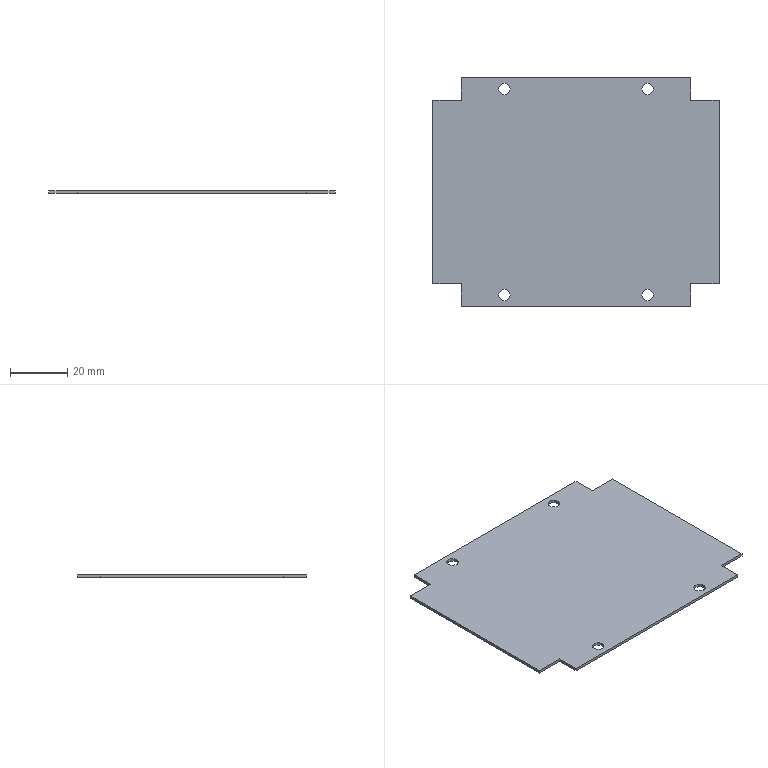Part | SolidWorks | features Extrusion 1 | 1 solid | 22 faces | box 100 x 80 x 1 mm | volume 7630 mm3 | plane 14 | cylinder 8 | commonest cylinder face diameters 4 x8
STEP:
#1=CARTESIAN_POINT('',(23.,-36.,1.));
#2=VERTEX_POINT('',#1);
#3=CARTESIAN_POINT('',(27.,-36.,1.));
#4=VERTEX_POINT('',#3);
#5=CARTESIAN_POINT('',(25.,-36.,1.));
#6=DIRECTION('',(0.,0.,1.));
#7=DIRECTION('',(1.,0.,0.));
#8=AXIS2_PLACEMENT_3D('',#5,#6,#7);
#9=CIRCLE('',#8,2.);
#10=EDGE_CURVE('',#2,#4,#9,.T.);
#11=ORIENTED_EDGE('',*,*,#10,.T.);
#12=CARTESIAN_POINT('',(27.,-36.,0.));
#13=VERTEX_POINT('',#12);
#14=CARTESIAN_POINT('',(27.,-36.,1.));
#15=DIRECTION('',(0.,0.,-1.));
#16=VECTOR('',#15,1000.);
#17=LINE('',#14,#16);
#18=EDGE_CURVE('',#4,#13,#17,.T.);
#19=ORIENTED_EDGE('',*,*,#18,.T.);
#20=CARTESIAN_POINT('',(23.,-36.,0.));
#21=VERTEX_POINT('',#20);
#22=CARTESIAN_POINT('',(25.,-36.,0.));
#23=DIRECTION('',(0.,0.,1.));
#24=DIRECTION('',(1.,0.,0.));
#25=AXIS2_PLACEMENT_3D('',#22,#23,#24);
#26=CIRCLE('',#25,2.);
#27=EDGE_CURVE('',#21,#13,#26,.T.);
#28=ORIENTED_EDGE('',*,*,#27,.F.);
#29=CARTESIAN_POINT('',(23.,-36.,1.));
#30=DIRECTION('',(0.,0.,-1.));
#31=VECTOR('',#30,1000.);
#32=LINE('',#29,#31);
#33=EDGE_CURVE('',#2,#21,#32,.T.);
#34=ORIENTED_EDGE('',*,*,#33,.F.);
#35=EDGE_LOOP('',(#11,#19,#28,#34));
#36=FACE_OUTER_BOUND('',#35,.T.);
#37=CARTESIAN_POINT('',(25.,-36.,1.));
#38=DIRECTION('',(0.,0.,-1.));
#39=DIRECTION('',(-1.,0.,0.));
#40=AXIS2_PLACEMENT_3D('',#37,#38,#39);
#41=CYLINDRICAL_SURFACE('',#40,2.);
#42=ADVANCED_FACE('',(#36),#41,.F.);
#43=CARTESIAN_POINT('',(23.,36.,1.));
#44=VERTEX_POINT('',#43);
#45=CARTESIAN_POINT('',(27.,36.,1.));
#46=VERTEX_POINT('',#45);
#47=CARTESIAN_POINT('',(25.,36.,1.));
#48=DIRECTION('',(0.,0.,1.));
#49=DIRECTION('',(1.,0.,0.));
#50=AXIS2_PLACEMENT_3D('',#47,#48,#49);
#51=CIRCLE('',#50,2.);
#52=EDGE_CURVE('',#44,#46,#51,.T.);
#53=ORIENTED_EDGE('',*,*,#52,.T.);
#54=CARTESIAN_POINT('',(27.,36.,0.));
#55=VERTEX_POINT('',#54);
#56=CARTESIAN_POINT('',(27.,36.,1.));
#57=DIRECTION('',(0.,0.,-1.));
#58=VECTOR('',#57,1000.);
#59=LINE('',#56,#58);
#60=EDGE_CURVE('',#46,#55,#59,.T.);
#61=ORIENTED_EDGE('',*,*,#60,.T.);
#62=CARTESIAN_POINT('',(23.,36.,0.));
#63=VERTEX_POINT('',#62);
#64=CARTESIAN_POINT('',(25.,36.,0.));
#65=DIRECTION('',(0.,0.,1.));
#66=DIRECTION('',(1.,0.,0.));
#67=AXIS2_PLACEMENT_3D('',#64,#65,#66);
#68=CIRCLE('',#67,2.);
#69=EDGE_CURVE('',#63,#55,#68,.T.);
#70=ORIENTED_EDGE('',*,*,#69,.F.);
#71=CARTESIAN_POINT('',(23.,36.,1.));
#72=DIRECTION('',(0.,0.,-1.));
#73=VECTOR('',#72,1000.);
#74=LINE('',#71,#73);
#75=EDGE_CURVE('',#44,#63,#74,.T.);
#76=ORIENTED_EDGE('',*,*,#75,.F.);
#77=EDGE_LOOP('',(#53,#61,#70,#76));
#78=FACE_OUTER_BOUND('',#77,.T.);
#79=CARTESIAN_POINT('',(25.,36.,1.));
#80=DIRECTION('',(0.,0.,-1.));
#81=DIRECTION('',(-1.,0.,0.));
#82=AXIS2_PLACEMENT_3D('',#79,#80,#81);
#83=CYLINDRICAL_SURFACE('',#82,2.);
#84=ADVANCED_FACE('',(#78),#83,.F.);
#85=CARTESIAN_POINT('',(-27.,-36.,1.));
#86=VERTEX_POINT('',#85);
#87=CARTESIAN_POINT('',(-23.,-36.,1.));
#88=VERTEX_POINT('',#87);
#89=CARTESIAN_POINT('',(-25.,-36.,1.));
#90=DIRECTION('',(0.,0.,1.));
#91=DIRECTION('',(1.,0.,0.));
#92=AXIS2_PLACEMENT_3D('',#89,#90,#91);
#93=CIRCLE('',#92,2.);
#94=EDGE_CURVE('',#86,#88,#93,.T.);
#95=ORIENTED_EDGE('',*,*,#94,.T.);
#96=CARTESIAN_POINT('',(-23.,-36.,0.));
#97=VERTEX_POINT('',#96);
#98=CARTESIAN_POINT('',(-23.,-36.,1.));
#99=DIRECTION('',(0.,0.,-1.));
#100=VECTOR('',#99,1000.);
#101=LINE('',#98,#100);
#102=EDGE_CURVE('',#88,#97,#101,.T.);
#103=ORIENTED_EDGE('',*,*,#102,.T.);
#104=CARTESIAN_POINT('',(-27.,-36.,0.));
#105=VERTEX_POINT('',#104);
#106=CARTESIAN_POINT('',(-25.,-36.,0.));
#107=DIRECTION('',(0.,0.,1.));
#108=DIRECTION('',(1.,0.,0.));
#109=AXIS2_PLACEMENT_3D('',#106,#107,#108);
#110=CIRCLE('',#109,2.);
#111=EDGE_CURVE('',#105,#97,#110,.T.);
#112=ORIENTED_EDGE('',*,*,#111,.F.);
#113=CARTESIAN_POINT('',(-27.,-36.,1.));
#114=DIRECTION('',(0.,0.,-1.));
#115=VECTOR('',#114,1000.);
#116=LINE('',#113,#115);
#117=EDGE_CURVE('',#86,#105,#116,.T.);
#118=ORIENTED_EDGE('',*,*,#117,.F.);
#119=EDGE_LOOP('',(#95,#103,#112,#118));
#120=FACE_OUTER_BOUND('',#119,.T.);
#121=CARTESIAN_POINT('',(-25.,-36.,1.));
#122=DIRECTION('',(0.,0.,-1.));
#123=DIRECTION('',(-1.,0.,0.));
#124=AXIS2_PLACEMENT_3D('',#121,#122,#123);
#125=CYLINDRICAL_SURFACE('',#124,2.);
#126=ADVANCED_FACE('',(#120),#125,.F.);
#127=CARTESIAN_POINT('',(-27.,36.,1.));
#128=VERTEX_POINT('',#127);
#129=CARTESIAN_POINT('',(-23.,36.,1.));
#130=VERTEX_POINT('',#129);
#131=CARTESIAN_POINT('',(-25.,36.,1.));
#132=DIRECTION('',(0.,0.,1.));
#133=DIRECTION('',(1.,0.,0.));
#134=AXIS2_PLACEMENT_3D('',#131,#132,#133);
#135=CIRCLE('',#134,2.);
#136=EDGE_CURVE('',#128,#130,#135,.T.);
#137=ORIENTED_EDGE('',*,*,#136,.T.);
#138=CARTESIAN_POINT('',(-23.,36.,0.));
#139=VERTEX_POINT('',#138);
#140=CARTESIAN_POINT('',(-23.,36.,1.));
#141=DIRECTION('',(0.,0.,-1.));
#142=VECTOR('',#141,1000.);
#143=LINE('',#140,#142);
#144=EDGE_CURVE('',#130,#139,#143,.T.);
#145=ORIENTED_EDGE('',*,*,#144,.T.);
#146=CARTESIAN_POINT('',(-27.,36.,0.));
#147=VERTEX_POINT('',#146);
#148=CARTESIAN_POINT('',(-25.,36.,0.));
#149=DIRECTION('',(0.,0.,1.));
#150=DIRECTION('',(1.,0.,0.));
#151=AXIS2_PLACEMENT_3D('',#148,#149,#150);
#152=CIRCLE('',#151,2.);
#153=EDGE_CURVE('',#147,#139,#152,.T.);
#154=ORIENTED_EDGE('',*,*,#153,.F.);
#155=CARTESIAN_POINT('',(-27.,36.,1.));
#156=DIRECTION('',(0.,0.,-1.));
#157=VECTOR('',#156,1000.);
#158=LINE('',#155,#157);
#159=EDGE_CURVE('',#128,#147,#158,.T.);
#160=ORIENTED_EDGE('',*,*,#159,.F.);
#161=EDGE_LOOP('',(#137,#145,#154,#160));
#162=FACE_OUTER_BOUND('',#161,.T.);
#163=CARTESIAN_POINT('',(-25.,36.,1.));
#164=DIRECTION('',(0.,0.,-1.));
#165=DIRECTION('',(-1.,0.,0.));
#166=AXIS2_PLACEMENT_3D('',#163,#164,#165);
#167=CYLINDRICAL_SURFACE('',#166,2.);
#168=ADVANCED_FACE('',(#162),#167,.F.);
#169=ORIENTED_EDGE('',*,*,#52,.F.);
#170=CARTESIAN_POINT('',(25.,36.,1.));
#171=DIRECTION('',(0.,0.,1.));
#172=DIRECTION('',(1.,0.,0.));
#173=AXIS2_PLACEMENT_3D('',#170,#171,#172);
#174=CIRCLE('',#173,2.);
#175=EDGE_CURVE('',#46,#44,#174,.T.);
#176=ORIENTED_EDGE('',*,*,#175,.F.);
#177=EDGE_LOOP('',(#169,#176));
#178=FACE_BOUND('',#177,.T.);
#179=ORIENTED_EDGE('',*,*,#136,.F.);
#180=CARTESIAN_POINT('',(-25.,36.,1.));
#181=DIRECTION('',(0.,0.,1.));
#182=DIRECTION('',(1.,0.,0.));
#183=AXIS2_PLACEMENT_3D('',#180,#181,#182);
#184=CIRCLE('',#183,2.);
#185=EDGE_CURVE('',#130,#128,#184,.T.);
#186=ORIENTED_EDGE('',*,*,#185,.F.);
#187=EDGE_LOOP('',(#179,#186));
#188=FACE_BOUND('',#187,.T.);
#189=CARTESIAN_POINT('',(-40.,32.,1.));
#190=VERTEX_POINT('',#189);
#191=CARTESIAN_POINT('',(-50.,32.,1.));
#192=VERTEX_POINT('',#191);
#193=CARTESIAN_POINT('',(-50.,32.,1.));
#194=DIRECTION('',(-1.,0.,0.));
#195=VECTOR('',#194,1000.);
#196=LINE('',#193,#195);
#197=EDGE_CURVE('',#190,#192,#196,.T.);
#198=ORIENTED_EDGE('',*,*,#197,.T.);
#199=CARTESIAN_POINT('',(-50.,-32.,1.));
#200=VERTEX_POINT('',#199);
#201=CARTESIAN_POINT('',(-50.,32.,1.));
#202=DIRECTION('',(0.,-1.,0.));
#203=VECTOR('',#202,1000.);
#204=LINE('',#201,#203);
#205=EDGE_CURVE('',#192,#200,#204,.T.);
#206=ORIENTED_EDGE('',*,*,#205,.T.);
#207=CARTESIAN_POINT('',(-40.,-32.,1.));
#208=VERTEX_POINT('',#207);
#209=CARTESIAN_POINT('',(-50.,-32.,1.));
#210=DIRECTION('',(1.,0.,0.));
#211=VECTOR('',#210,1000.);
#212=LINE('',#209,#211);
#213=EDGE_CURVE('',#200,#208,#212,.T.);
#214=ORIENTED_EDGE('',*,*,#213,.T.);
#215=CARTESIAN_POINT('',(-40.,-40.,1.));
#216=VERTEX_POINT('',#215);
#217=CARTESIAN_POINT('',(-40.,-32.,1.));
#218=DIRECTION('',(0.,-1.,0.));
#219=VECTOR('',#218,1000.);
#220=LINE('',#217,#219);
#221=EDGE_CURVE('',#208,#216,#220,.T.);
#222=ORIENTED_EDGE('',*,*,#221,.T.);
#223=CARTESIAN_POINT('',(40.,-40.,1.));
#224=VERTEX_POINT('',#223);
#225=CARTESIAN_POINT('',(-40.,-40.,1.));
#226=DIRECTION('',(1.,0.,0.));
#227=VECTOR('',#226,1000.);
#228=LINE('',#225,#227);
#229=EDGE_CURVE('',#216,#224,#228,.T.);
#230=ORIENTED_EDGE('',*,*,#229,.T.);
#231=CARTESIAN_POINT('',(40.,-32.,1.));
#232=VERTEX_POINT('',#231);
#233=CARTESIAN_POINT('',(40.,-32.,1.));
#234=DIRECTION('',(0.,1.,0.));
#235=VECTOR('',#234,1000.);
#236=LINE('',#233,#235);
#237=EDGE_CURVE('',#224,#232,#236,.T.);
#238=ORIENTED_EDGE('',*,*,#237,.T.);
#239=CARTESIAN_POINT('',(50.,-32.,1.));
#240=VERTEX_POINT('',#239);
#241=CARTESIAN_POINT('',(50.,-32.,1.));
#242=DIRECTION('',(1.,0.,0.));
#243=VECTOR('',#242,1000.);
#244=LINE('',#241,#243);
#245=EDGE_CURVE('',#232,#240,#244,.T.);
#246=ORIENTED_EDGE('',*,*,#245,.T.);
#247=CARTESIAN_POINT('',(50.,32.,1.));
#248=VERTEX_POINT('',#247);
#249=CARTESIAN_POINT('',(50.,32.,1.));
#250=DIRECTION('',(0.,1.,0.));
#251=VECTOR('',#250,1000.);
#252=LINE('',#249,#251);
#253=EDGE_CURVE('',#240,#248,#252,.T.);
#254=ORIENTED_EDGE('',*,*,#253,.T.);
#255=CARTESIAN_POINT('',(40.,32.,1.));
#256=VERTEX_POINT('',#255);
#257=CARTESIAN_POINT('',(50.,32.,1.));
#258=DIRECTION('',(-1.,0.,0.));
#259=VECTOR('',#258,1000.);
#260=LINE('',#257,#259);
#261=EDGE_CURVE('',#248,#256,#260,.T.);
#262=ORIENTED_EDGE('',*,*,#261,.T.);
#263=CARTESIAN_POINT('',(40.,40.,1.));
#264=VERTEX_POINT('',#263);
#265=CARTESIAN_POINT('',(40.,32.,1.));
#266=DIRECTION('',(0.,1.,0.));
#267=VECTOR('',#266,1000.);
#268=LINE('',#265,#267);
#269=EDGE_CURVE('',#256,#264,#268,.T.);
#270=ORIENTED_EDGE('',*,*,#269,.T.);
#271=CARTESIAN_POINT('',(-40.,40.,1.));
#272=VERTEX_POINT('',#271);
#273=CARTESIAN_POINT('',(-40.,40.,1.));
#274=DIRECTION('',(-1.,0.,0.));
#275=VECTOR('',#274,1000.);
#276=LINE('',#273,#275);
#277=EDGE_CURVE('',#264,#272,#276,.T.);
#278=ORIENTED_EDGE('',*,*,#277,.T.);
#279=CARTESIAN_POINT('',(-40.,32.,1.));
#280=DIRECTION('',(0.,-1.,0.));
#281=VECTOR('',#280,1000.);
#282=LINE('',#279,#281);
#283=EDGE_CURVE('',#272,#190,#282,.T.);
#284=ORIENTED_EDGE('',*,*,#283,.T.);
#285=EDGE_LOOP('',(#198,#206,#214,#222,#230,#238,#246,#254,#262,#270,#278,#284));
#286=FACE_OUTER_BOUND('',#285,.T.);
#287=ORIENTED_EDGE('',*,*,#94,.F.);
#288=CARTESIAN_POINT('',(-25.,-36.,1.));
#289=DIRECTION('',(0.,0.,1.));
#290=DIRECTION('',(1.,0.,0.));
#291=AXIS2_PLACEMENT_3D('',#288,#289,#290);
#292=CIRCLE('',#291,2.);
#293=EDGE_CURVE('',#88,#86,#292,.T.);
#294=ORIENTED_EDGE('',*,*,#293,.F.);
#295=EDGE_LOOP('',(#287,#294));
#296=FACE_BOUND('',#295,.T.);
#297=ORIENTED_EDGE('',*,*,#10,.F.);
#298=CARTESIAN_POINT('',(25.,-36.,1.));
#299=DIRECTION('',(0.,0.,1.));
#300=DIRECTION('',(1.,0.,0.));
#301=AXIS2_PLACEMENT_3D('',#298,#299,#300);
#302=CIRCLE('',#301,2.);
#303=EDGE_CURVE('',#4,#2,#302,.T.);
#304=ORIENTED_EDGE('',*,*,#303,.F.);
#305=EDGE_LOOP('',(#297,#304));
#306=FACE_BOUND('',#305,.T.);
#307=CARTESIAN_POINT('',(0.,0.,1.));
#308=DIRECTION('',(0.,0.,1.));
#309=DIRECTION('',(1.,0.,0.));
#310=AXIS2_PLACEMENT_3D('',#307,#308,#309);
#311=PLANE('',#310);
#312=ADVANCED_FACE('',(#178,#188,#286,#296,#306),#311,.T.);
#313=CARTESIAN_POINT('',(-40.,32.,0.));
#314=VERTEX_POINT('',#313);
#315=CARTESIAN_POINT('',(-50.,32.,0.));
#316=VERTEX_POINT('',#315);
#317=CARTESIAN_POINT('',(-50.,32.,0.));
#318=DIRECTION('',(-1.,0.,0.));
#319=VECTOR('',#318,1000.);
#320=LINE('',#317,#319);
#321=EDGE_CURVE('',#314,#316,#320,.T.);
#322=ORIENTED_EDGE('',*,*,#321,.F.);
#323=CARTESIAN_POINT('',(-40.,40.,0.));
#324=VERTEX_POINT('',#323);
#325=CARTESIAN_POINT('',(-40.,32.,0.));
#326=DIRECTION('',(0.,-1.,0.));
#327=VECTOR('',#326,1000.);
#328=LINE('',#325,#327);
#329=EDGE_CURVE('',#324,#314,#328,.T.);
#330=ORIENTED_EDGE('',*,*,#329,.F.);
#331=CARTESIAN_POINT('',(40.,40.,0.));
#332=VERTEX_POINT('',#331);
#333=CARTESIAN_POINT('',(-40.,40.,0.));
#334=DIRECTION('',(-1.,0.,0.));
#335=VECTOR('',#334,1000.);
#336=LINE('',#333,#335);
#337=EDGE_CURVE('',#332,#324,#336,.T.);
#338=ORIENTED_EDGE('',*,*,#337,.F.);
#339=CARTESIAN_POINT('',(40.,32.,0.));
#340=VERTEX_POINT('',#339);
#341=CARTESIAN_POINT('',(40.,32.,0.));
#342=DIRECTION('',(0.,1.,0.));
#343=VECTOR('',#342,1000.);
#344=LINE('',#341,#343);
#345=EDGE_CURVE('',#340,#332,#344,.T.);
#346=ORIENTED_EDGE('',*,*,#345,.F.);
#347=CARTESIAN_POINT('',(50.,32.,0.));
#348=VERTEX_POINT('',#347);
#349=CARTESIAN_POINT('',(50.,32.,0.));
#350=DIRECTION('',(-1.,0.,0.));
#351=VECTOR('',#350,1000.);
#352=LINE('',#349,#351);
#353=EDGE_CURVE('',#348,#340,#352,.T.);
#354=ORIENTED_EDGE('',*,*,#353,.F.);
#355=CARTESIAN_POINT('',(50.,-32.,0.));
#356=VERTEX_POINT('',#355);
#357=CARTESIAN_POINT('',(50.,32.,0.));
#358=DIRECTION('',(0.,1.,0.));
#359=VECTOR('',#358,1000.);
#360=LINE('',#357,#359);
#361=EDGE_CURVE('',#356,#348,#360,.T.);
#362=ORIENTED_EDGE('',*,*,#361,.F.);
#363=CARTESIAN_POINT('',(40.,-32.,0.));
#364=VERTEX_POINT('',#363);
#365=CARTESIAN_POINT('',(50.,-32.,0.));
#366=DIRECTION('',(1.,0.,0.));
#367=VECTOR('',#366,1000.);
#368=LINE('',#365,#367);
#369=EDGE_CURVE('',#364,#356,#368,.T.);
#370=ORIENTED_EDGE('',*,*,#369,.F.);
#371=CARTESIAN_POINT('',(40.,-40.,0.));
#372=VERTEX_POINT('',#371);
#373=CARTESIAN_POINT('',(40.,-32.,0.));
#374=DIRECTION('',(0.,1.,0.));
#375=VECTOR('',#374,1000.);
#376=LINE('',#373,#375);
#377=EDGE_CURVE('',#372,#364,#376,.T.);
#378=ORIENTED_EDGE('',*,*,#377,.F.);
#379=CARTESIAN_POINT('',(-40.,-40.,0.));
#380=VERTEX_POINT('',#379);
#381=CARTESIAN_POINT('',(-40.,-40.,0.));
#382=DIRECTION('',(1.,0.,0.));
#383=VECTOR('',#382,1000.);
#384=LINE('',#381,#383);
#385=EDGE_CURVE('',#380,#372,#384,.T.);
#386=ORIENTED_EDGE('',*,*,#385,.F.);
#387=CARTESIAN_POINT('',(-40.,-32.,0.));
#388=VERTEX_POINT('',#387);
#389=CARTESIAN_POINT('',(-40.,-32.,0.));
#390=DIRECTION('',(0.,-1.,0.));
#391=VECTOR('',#390,1000.);
#392=LINE('',#389,#391);
#393=EDGE_CURVE('',#388,#380,#392,.T.);
#394=ORIENTED_EDGE('',*,*,#393,.F.);
#395=CARTESIAN_POINT('',(-50.,-32.,0.));
#396=VERTEX_POINT('',#395);
#397=CARTESIAN_POINT('',(-50.,-32.,0.));
#398=DIRECTION('',(1.,0.,0.));
#399=VECTOR('',#398,1000.);
#400=LINE('',#397,#399);
#401=EDGE_CURVE('',#396,#388,#400,.T.);
#402=ORIENTED_EDGE('',*,*,#401,.F.);
#403=CARTESIAN_POINT('',(-50.,32.,0.));
#404=DIRECTION('',(0.,-1.,0.));
#405=VECTOR('',#404,1000.);
#406=LINE('',#403,#405);
#407=EDGE_CURVE('',#316,#396,#406,.T.);
#408=ORIENTED_EDGE('',*,*,#407,.F.);
#409=EDGE_LOOP('',(#322,#330,#338,#346,#354,#362,#370,#378,#386,#394,#402,#408));
#410=FACE_OUTER_BOUND('',#409,.T.);
#411=ORIENTED_EDGE('',*,*,#153,.T.);
#412=CARTESIAN_POINT('',(-25.,36.,0.));
#413=DIRECTION('',(0.,0.,1.));
#414=DIRECTION('',(1.,0.,0.));
#415=AXIS2_PLACEMENT_3D('',#412,#413,#414);
#416=CIRCLE('',#415,2.);
#417=EDGE_CURVE('',#139,#147,#416,.T.);
#418=ORIENTED_EDGE('',*,*,#417,.T.);
#419=EDGE_LOOP('',(#411,#418));
#420=FACE_BOUND('',#419,.T.);
#421=ORIENTED_EDGE('',*,*,#111,.T.);
#422=CARTESIAN_POINT('',(-25.,-36.,0.));
#423=DIRECTION('',(0.,0.,1.));
#424=DIRECTION('',(1.,0.,0.));
#425=AXIS2_PLACEMENT_3D('',#422,#423,#424);
#426=CIRCLE('',#425,2.);
#427=EDGE_CURVE('',#97,#105,#426,.T.);
#428=ORIENTED_EDGE('',*,*,#427,.T.);
#429=EDGE_LOOP('',(#421,#428));
#430=FACE_BOUND('',#429,.T.);
#431=ORIENTED_EDGE('',*,*,#69,.T.);
#432=CARTESIAN_POINT('',(25.,36.,0.));
#433=DIRECTION('',(0.,0.,1.));
#434=DIRECTION('',(1.,0.,0.));
#435=AXIS2_PLACEMENT_3D('',#432,#433,#434);
#436=CIRCLE('',#435,2.);
#437=EDGE_CURVE('',#55,#63,#436,.T.);
#438=ORIENTED_EDGE('',*,*,#437,.T.);
#439=EDGE_LOOP('',(#431,#438));
#440=FACE_BOUND('',#439,.T.);
#441=ORIENTED_EDGE('',*,*,#27,.T.);
#442=CARTESIAN_POINT('',(25.,-36.,0.));
#443=DIRECTION('',(0.,0.,1.));
#444=DIRECTION('',(1.,0.,0.));
#445=AXIS2_PLACEMENT_3D('',#442,#443,#444);
#446=CIRCLE('',#445,2.);
#447=EDGE_CURVE('',#13,#21,#446,.T.);
#448=ORIENTED_EDGE('',*,*,#447,.T.);
#449=EDGE_LOOP('',(#441,#448));
#450=FACE_BOUND('',#449,.T.);
#451=CARTESIAN_POINT('',(0.,0.,0.));
#452=DIRECTION('',(0.,0.,1.));
#453=DIRECTION('',(1.,0.,0.));
#454=AXIS2_PLACEMENT_3D('',#451,#452,#453);
#455=PLANE('',#454);
#456=ADVANCED_FACE('',(#410,#420,#430,#440,#450),#455,.F.);
#457=ORIENTED_EDGE('',*,*,#321,.T.);
#458=CARTESIAN_POINT('',(-50.,32.,1.));
#459=DIRECTION('',(0.,0.,-1.));
#460=VECTOR('',#459,1000.);
#461=LINE('',#458,#460);
#462=EDGE_CURVE('',#192,#316,#461,.T.);
#463=ORIENTED_EDGE('',*,*,#462,.F.);
#464=ORIENTED_EDGE('',*,*,#197,.F.);
#465=CARTESIAN_POINT('',(-40.,32.,1.));
#466=DIRECTION('',(0.,0.,-1.));
#467=VECTOR('',#466,1000.);
#468=LINE('',#465,#467);
#469=EDGE_CURVE('',#190,#314,#468,.T.);
#470=ORIENTED_EDGE('',*,*,#469,.T.);
#471=EDGE_LOOP('',(#457,#463,#464,#470));
#472=FACE_OUTER_BOUND('',#471,.T.);
#473=CARTESIAN_POINT('',(-50.,32.,1.));
#474=DIRECTION('',(0.,-1.,0.));
#475=DIRECTION('',(0.,0.,-1.));
#476=AXIS2_PLACEMENT_3D('',#473,#474,#475);
#477=PLANE('',#476);
#478=ADVANCED_FACE('',(#472),#477,.F.);
#479=ORIENTED_EDGE('',*,*,#407,.T.);
#480=CARTESIAN_POINT('',(-50.,-32.,1.));
#481=DIRECTION('',(0.,0.,-1.));
#482=VECTOR('',#481,1000.);
#483=LINE('',#480,#482);
#484=EDGE_CURVE('',#200,#396,#483,.T.);
#485=ORIENTED_EDGE('',*,*,#484,.F.);
#486=ORIENTED_EDGE('',*,*,#205,.F.);
#487=ORIENTED_EDGE('',*,*,#462,.T.);
#488=EDGE_LOOP('',(#479,#485,#486,#487));
#489=FACE_OUTER_BOUND('',#488,.T.);
#490=CARTESIAN_POINT('',(-50.,32.,1.));
#491=DIRECTION('',(1.,0.,0.));
#492=DIRECTION('',(0.,1.,0.));
#493=AXIS2_PLACEMENT_3D('',#490,#491,#492);
#494=PLANE('',#493);
#495=ADVANCED_FACE('',(#489),#494,.F.);
#496=ORIENTED_EDGE('',*,*,#401,.T.);
#497=CARTESIAN_POINT('',(-40.,-32.,1.));
#498=DIRECTION('',(0.,0.,-1.));
#499=VECTOR('',#498,1000.);
#500=LINE('',#497,#499);
#501=EDGE_CURVE('',#208,#388,#500,.T.);
#502=ORIENTED_EDGE('',*,*,#501,.F.);
#503=ORIENTED_EDGE('',*,*,#213,.F.);
#504=ORIENTED_EDGE('',*,*,#484,.T.);
#505=EDGE_LOOP('',(#496,#502,#503,#504));
#506=FACE_OUTER_BOUND('',#505,.T.);
#507=CARTESIAN_POINT('',(-50.,-32.,1.));
#508=DIRECTION('',(0.,1.,0.));
#509=DIRECTION('',(-1.,0.,0.));
#510=AXIS2_PLACEMENT_3D('',#507,#508,#509);
#511=PLANE('',#510);
#512=ADVANCED_FACE('',(#506),#511,.F.);
#513=ORIENTED_EDGE('',*,*,#393,.T.);
#514=CARTESIAN_POINT('',(-40.,-40.,1.));
#515=DIRECTION('',(0.,0.,-1.));
#516=VECTOR('',#515,1000.);
#517=LINE('',#514,#516);
#518=EDGE_CURVE('',#216,#380,#517,.T.);
#519=ORIENTED_EDGE('',*,*,#518,.F.);
#520=ORIENTED_EDGE('',*,*,#221,.F.);
#521=ORIENTED_EDGE('',*,*,#501,.T.);
#522=EDGE_LOOP('',(#513,#519,#520,#521));
#523=FACE_OUTER_BOUND('',#522,.T.);
#524=CARTESIAN_POINT('',(-40.,-32.,1.));
#525=DIRECTION('',(1.,0.,0.));
#526=DIRECTION('',(0.,1.,0.));
#527=AXIS2_PLACEMENT_3D('',#524,#525,#526);
#528=PLANE('',#527);
#529=ADVANCED_FACE('',(#523),#528,.F.);
#530=ORIENTED_EDGE('',*,*,#385,.T.);
#531=CARTESIAN_POINT('',(40.,-40.,1.));
#532=DIRECTION('',(0.,0.,-1.));
#533=VECTOR('',#532,1000.);
#534=LINE('',#531,#533);
#535=EDGE_CURVE('',#224,#372,#534,.T.);
#536=ORIENTED_EDGE('',*,*,#535,.F.);
#537=ORIENTED_EDGE('',*,*,#229,.F.);
#538=ORIENTED_EDGE('',*,*,#518,.T.);
#539=EDGE_LOOP('',(#530,#536,#537,#538));
#540=FACE_OUTER_BOUND('',#539,.T.);
#541=CARTESIAN_POINT('',(-40.,-40.,1.));
#542=DIRECTION('',(0.,1.,0.));
#543=DIRECTION('',(0.,0.,1.));
#544=AXIS2_PLACEMENT_3D('',#541,#542,#543);
#545=PLANE('',#544);
#546=ADVANCED_FACE('',(#540),#545,.F.);
#547=ORIENTED_EDGE('',*,*,#377,.T.);
#548=CARTESIAN_POINT('',(40.,-32.,1.));
#549=DIRECTION('',(0.,0.,-1.));
#550=VECTOR('',#549,1000.);
#551=LINE('',#548,#550);
#552=EDGE_CURVE('',#232,#364,#551,.T.);
#553=ORIENTED_EDGE('',*,*,#552,.F.);
#554=ORIENTED_EDGE('',*,*,#237,.F.);
#555=ORIENTED_EDGE('',*,*,#535,.T.);
#556=EDGE_LOOP('',(#547,#553,#554,#555));
#557=FACE_OUTER_BOUND('',#556,.T.);
#558=CARTESIAN_POINT('',(40.,-32.,1.));
#559=DIRECTION('',(-1.,0.,0.));
#560=DIRECTION('',(0.,-1.,0.));
#561=AXIS2_PLACEMENT_3D('',#558,#559,#560);
#562=PLANE('',#561);
#563=ADVANCED_FACE('',(#557),#562,.F.);
#564=ORIENTED_EDGE('',*,*,#369,.T.);
#565=CARTESIAN_POINT('',(50.,-32.,1.));
#566=DIRECTION('',(0.,0.,-1.));
#567=VECTOR('',#566,1000.);
#568=LINE('',#565,#567);
#569=EDGE_CURVE('',#240,#356,#568,.T.);
#570=ORIENTED_EDGE('',*,*,#569,.F.);
#571=ORIENTED_EDGE('',*,*,#245,.F.);
#572=ORIENTED_EDGE('',*,*,#552,.T.);
#573=EDGE_LOOP('',(#564,#570,#571,#572));
#574=FACE_OUTER_BOUND('',#573,.T.);
#575=CARTESIAN_POINT('',(50.,-32.,1.));
#576=DIRECTION('',(0.,1.,0.));
#577=DIRECTION('',(-1.,0.,0.));
#578=AXIS2_PLACEMENT_3D('',#575,#576,#577);
#579=PLANE('',#578);
#580=ADVANCED_FACE('',(#574),#579,.F.);
#581=ORIENTED_EDGE('',*,*,#361,.T.);
#582=CARTESIAN_POINT('',(50.,32.,1.));
#583=DIRECTION('',(0.,0.,-1.));
#584=VECTOR('',#583,1000.);
#585=LINE('',#582,#584);
#586=EDGE_CURVE('',#248,#348,#585,.T.);
#587=ORIENTED_EDGE('',*,*,#586,.F.);
#588=ORIENTED_EDGE('',*,*,#253,.F.);
#589=ORIENTED_EDGE('',*,*,#569,.T.);
#590=EDGE_LOOP('',(#581,#587,#588,#589));
#591=FACE_OUTER_BOUND('',#590,.T.);
#592=CARTESIAN_POINT('',(50.,32.,1.));
#593=DIRECTION('',(-1.,0.,0.));
#594=DIRECTION('',(0.,-1.,0.));
#595=AXIS2_PLACEMENT_3D('',#592,#593,#594);
#596=PLANE('',#595);
#597=ADVANCED_FACE('',(#591),#596,.F.);
#598=ORIENTED_EDGE('',*,*,#353,.T.);
#599=CARTESIAN_POINT('',(40.,32.,1.));
#600=DIRECTION('',(0.,0.,-1.));
#601=VECTOR('',#600,1000.);
#602=LINE('',#599,#601);
#603=EDGE_CURVE('',#256,#340,#602,.T.);
#604=ORIENTED_EDGE('',*,*,#603,.F.);
#605=ORIENTED_EDGE('',*,*,#261,.F.);
#606=ORIENTED_EDGE('',*,*,#586,.T.);
#607=EDGE_LOOP('',(#598,#604,#605,#606));
#608=FACE_OUTER_BOUND('',#607,.T.);
#609=CARTESIAN_POINT('',(50.,32.,1.));
#610=DIRECTION('',(0.,-1.,0.));
#611=DIRECTION('',(0.,0.,-1.));
#612=AXIS2_PLACEMENT_3D('',#609,#610,#611);
#613=PLANE('',#612);
#614=ADVANCED_FACE('',(#608),#613,.F.);
#615=ORIENTED_EDGE('',*,*,#345,.T.);
#616=CARTESIAN_POINT('',(40.,40.,1.));
#617=DIRECTION('',(0.,0.,-1.));
#618=VECTOR('',#617,1000.);
#619=LINE('',#616,#618);
#620=EDGE_CURVE('',#264,#332,#619,.T.);
#621=ORIENTED_EDGE('',*,*,#620,.F.);
#622=ORIENTED_EDGE('',*,*,#269,.F.);
#623=ORIENTED_EDGE('',*,*,#603,.T.);
#624=EDGE_LOOP('',(#615,#621,#622,#623));
#625=FACE_OUTER_BOUND('',#624,.T.);
#626=CARTESIAN_POINT('',(40.,32.,1.));
#627=DIRECTION('',(-1.,0.,0.));
#628=DIRECTION('',(0.,0.,1.));
#629=AXIS2_PLACEMENT_3D('',#626,#627,#628);
#630=PLANE('',#629);
#631=ADVANCED_FACE('',(#625),#630,.F.);
#632=ORIENTED_EDGE('',*,*,#337,.T.);
#633=CARTESIAN_POINT('',(-40.,40.,1.));
#634=DIRECTION('',(0.,0.,-1.));
#635=VECTOR('',#634,1000.);
#636=LINE('',#633,#635);
#637=EDGE_CURVE('',#272,#324,#636,.T.);
#638=ORIENTED_EDGE('',*,*,#637,.F.);
#639=ORIENTED_EDGE('',*,*,#277,.F.);
#640=ORIENTED_EDGE('',*,*,#620,.T.);
#641=EDGE_LOOP('',(#632,#638,#639,#640));
#642=FACE_OUTER_BOUND('',#641,.T.);
#643=CARTESIAN_POINT('',(-40.,40.,1.));
#644=DIRECTION('',(0.,-1.,0.));
#645=DIRECTION('',(0.,0.,-1.));
#646=AXIS2_PLACEMENT_3D('',#643,#644,#645);
#647=PLANE('',#646);
#648=ADVANCED_FACE('',(#642),#647,.F.);
#649=ORIENTED_EDGE('',*,*,#329,.T.);
#650=ORIENTED_EDGE('',*,*,#469,.F.);
#651=ORIENTED_EDGE('',*,*,#283,.F.);
#652=ORIENTED_EDGE('',*,*,#637,.T.);
#653=EDGE_LOOP('',(#649,#650,#651,#652));
#654=FACE_OUTER_BOUND('',#653,.T.);
#655=CARTESIAN_POINT('',(-40.,32.,1.));
#656=DIRECTION('',(1.,0.,0.));
#657=DIRECTION('',(0.,0.,-1.));
#658=AXIS2_PLACEMENT_3D('',#655,#656,#657);
#659=PLANE('',#658);
#660=ADVANCED_FACE('',(#654),#659,.F.);
#661=ORIENTED_EDGE('',*,*,#144,.F.);
#662=ORIENTED_EDGE('',*,*,#185,.T.);
#663=ORIENTED_EDGE('',*,*,#159,.T.);
#664=ORIENTED_EDGE('',*,*,#417,.F.);
#665=EDGE_LOOP('',(#661,#662,#663,#664));
#666=FACE_OUTER_BOUND('',#665,.T.);
#667=CARTESIAN_POINT('',(-25.,36.,1.));
#668=DIRECTION('',(0.,0.,-1.));
#669=DIRECTION('',(-1.,0.,0.));
#670=AXIS2_PLACEMENT_3D('',#667,#668,#669);
#671=CYLINDRICAL_SURFACE('',#670,2.);
#672=ADVANCED_FACE('',(#666),#671,.F.);
#673=ORIENTED_EDGE('',*,*,#102,.F.);
#674=ORIENTED_EDGE('',*,*,#293,.T.);
#675=ORIENTED_EDGE('',*,*,#117,.T.);
#676=ORIENTED_EDGE('',*,*,#427,.F.);
#677=EDGE_LOOP('',(#673,#674,#675,#676));
#678=FACE_OUTER_BOUND('',#677,.T.);
#679=CARTESIAN_POINT('',(-25.,-36.,1.));
#680=DIRECTION('',(0.,0.,-1.));
#681=DIRECTION('',(-1.,0.,0.));
#682=AXIS2_PLACEMENT_3D('',#679,#680,#681);
#683=CYLINDRICAL_SURFACE('',#682,2.);
#684=ADVANCED_FACE('',(#678),#683,.F.);
#685=ORIENTED_EDGE('',*,*,#60,.F.);
#686=ORIENTED_EDGE('',*,*,#175,.T.);
#687=ORIENTED_EDGE('',*,*,#75,.T.);
#688=ORIENTED_EDGE('',*,*,#437,.F.);
#689=EDGE_LOOP('',(#685,#686,#687,#688));
#690=FACE_OUTER_BOUND('',#689,.T.);
#691=CARTESIAN_POINT('',(25.,36.,1.));
#692=DIRECTION('',(0.,0.,-1.));
#693=DIRECTION('',(-1.,0.,0.));
#694=AXIS2_PLACEMENT_3D('',#691,#692,#693);
#695=CYLINDRICAL_SURFACE('',#694,2.);
#696=ADVANCED_FACE('',(#690),#695,.F.);
#697=ORIENTED_EDGE('',*,*,#18,.F.);
#698=ORIENTED_EDGE('',*,*,#303,.T.);
#699=ORIENTED_EDGE('',*,*,#33,.T.);
#700=ORIENTED_EDGE('',*,*,#447,.F.);
#701=EDGE_LOOP('',(#697,#698,#699,#700));
#702=FACE_OUTER_BOUND('',#701,.T.);
#703=CARTESIAN_POINT('',(25.,-36.,1.));
#704=DIRECTION('',(0.,0.,-1.));
#705=DIRECTION('',(-1.,0.,0.));
#706=AXIS2_PLACEMENT_3D('',#703,#704,#705);
#707=CYLINDRICAL_SURFACE('',#706,2.);
#708=ADVANCED_FACE('',(#702),#707,.F.);
#709=CLOSED_SHELL('',(#42,#84,#126,#168,#312,#456,#478,#495,#512,#529,#546,#563,#580,#597,#614,#631,#648,#660,#672,#684,#696,#708));
#710=MANIFOLD_SOLID_BREP('',#709);
#711=CARTESIAN_POINT('',(0.,0.,0.));
#712=DIRECTION('',(0.,0.,1.));
#713=DIRECTION('',(1.,0.,0.));
#714=AXIS2_PLACEMENT_3D('',#711,#712,#713);
#715=(LENGTH_UNIT()NAMED_UNIT(*)SI_UNIT(.MILLI.,.METRE.));
#716=UNCERTAINTY_MEASURE_WITH_UNIT(LENGTH_MEASURE(0.00001),#715,'','');
#717=(NAMED_UNIT(*)PLANE_ANGLE_UNIT()SI_UNIT($,.RADIAN.));
#718=(NAMED_UNIT(*)SI_UNIT($,.STERADIAN.)SOLID_ANGLE_UNIT());
#719=(GEOMETRIC_REPRESENTATION_CONTEXT(3)GLOBAL_UNCERTAINTY_ASSIGNED_CONTEXT((#716))GLOBAL_UNIT_ASSIGNED_CONTEXT((#715,#717,#718))REPRESENTATION_CONTEXT('',''));
#720=ADVANCED_BREP_SHAPE_REPRESENTATION('',(#710,#714),#719);